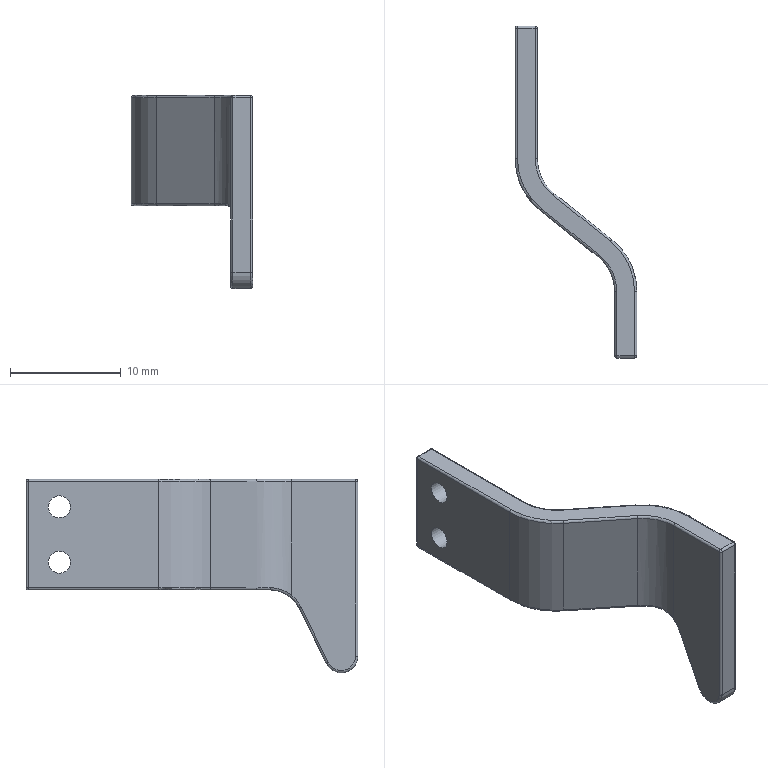Part | STEP file | 1-04.5 | 1 solid | 58 faces | box 11 x 30 x 17.5 mm | volume 723.407 mm3 | cylinder 27 | torus 12 | plane 11 | sphere 6 | spline 2 | commonest cylinder face diameters 0.4 x19 2 x2 8 x2 12 x2 3 x1 6 x1